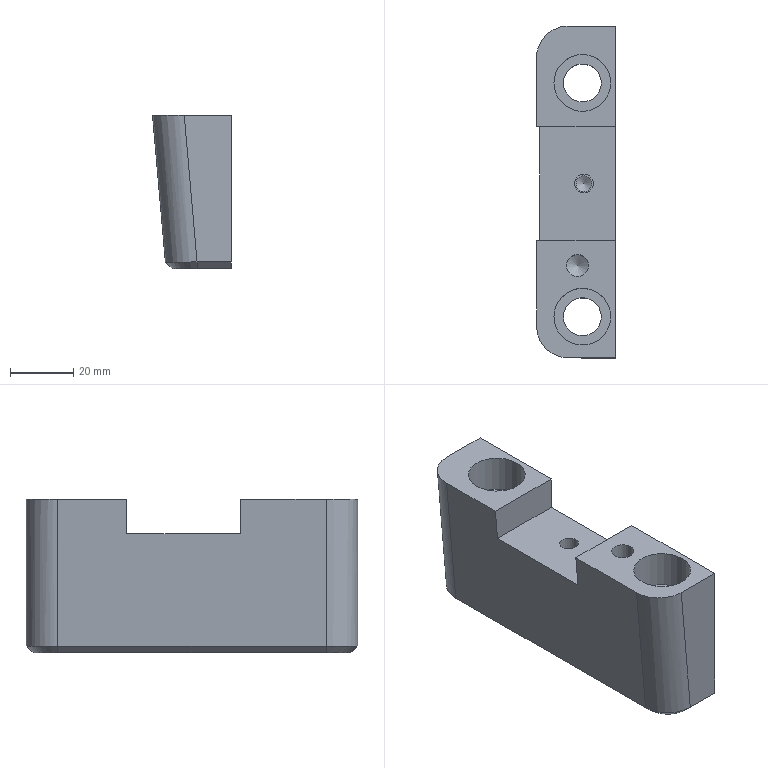Part | STEP file | solid 80 | 1 solid | 29 faces | box 25 x 105 x 48.598 mm | volume 89141 mm3 | plane 16 | cylinder 9 | cone 2 | spline 2 | commonest cylinder face diameters 12 x2 18 x2 20 x2 5 x1 6 x1 7 x1